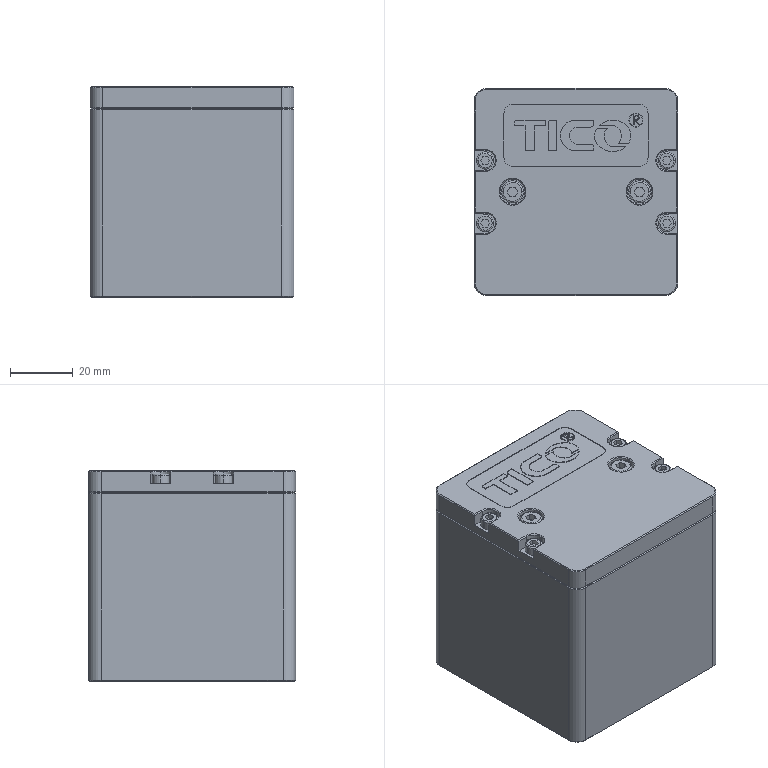Part | SolidWorks | features BaseBody 3 | 3 solids | 433 faces | box 65 x 66.1 x 67 mm | volume 277180 mm3 | plane 218 | cylinder 114 | cone 80 | spline 21 | commonest cylinder face diameters 6 x18 5.5 x16 8 x12 10 x10 3.3 x8 3.4 x8